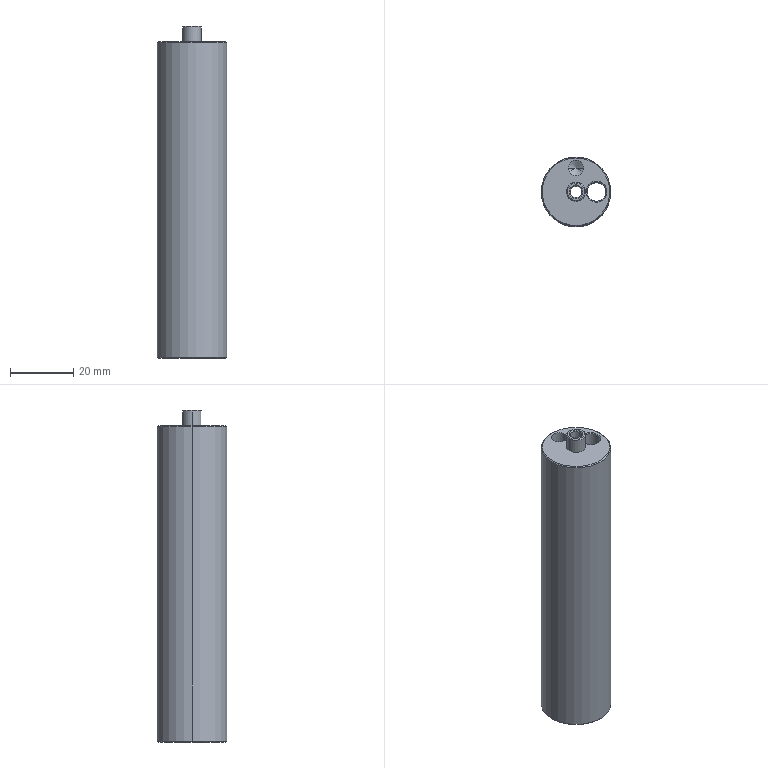Part | SolidWorks | features ICE 3, Chamfer 1, Extrusion 1, HoleWzd 1 | 1 solid | 29 faces | box 22 x 22 x 105 mm | volume 33982 mm3 | cone 16 | cylinder 10 | plane 3 | commonest cylinder face diameters 6 x4 3.7 x2 5 x2 22 x2
STEP:
#1=CARTESIAN_POINT('',(10.7,0.,100.));
#2=VERTEX_POINT('',#1);
#3=CARTESIAN_POINT('',(-10.7,0.,100.));
#4=VERTEX_POINT('',#3);
#5=CARTESIAN_POINT('',(0.,0.,100.));
#6=DIRECTION('',(0.,0.,1.));
#7=DIRECTION('',(1.,0.,0.));
#8=AXIS2_PLACEMENT_3D('',#5,#6,#7);
#9=CIRCLE('',#8,10.7);
#10=EDGE_CURVE('',#2,#4,#9,.T.);
#11=ORIENTED_EDGE('',*,*,#10,.F.);
#12=CARTESIAN_POINT('',(11.,0.,99.7));
#13=VERTEX_POINT('',#12);
#14=CARTESIAN_POINT('',(10.7,0.,100.));
#15=DIRECTION('',(0.7071,0.,-0.7071));
#16=VECTOR('',#15,1000.);
#17=LINE('',#14,#16);
#18=EDGE_CURVE('',#2,#13,#17,.T.);
#19=ORIENTED_EDGE('',*,*,#18,.T.);
#20=CARTESIAN_POINT('',(-11.,0.,99.7));
#21=VERTEX_POINT('',#20);
#22=CARTESIAN_POINT('',(0.,0.,99.7));
#23=DIRECTION('',(0.,0.,-1.));
#24=DIRECTION('',(1.,0.,0.));
#25=AXIS2_PLACEMENT_3D('',#22,#23,#24);
#26=CIRCLE('',#25,11.);
#27=EDGE_CURVE('',#21,#13,#26,.T.);
#28=ORIENTED_EDGE('',*,*,#27,.F.);
#29=CARTESIAN_POINT('',(-10.7,0.,100.));
#30=DIRECTION('',(-0.7071,0.,-0.7071));
#31=VECTOR('',#30,1000.);
#32=LINE('',#29,#31);
#33=EDGE_CURVE('',#4,#21,#32,.T.);
#34=ORIENTED_EDGE('',*,*,#33,.F.);
#35=EDGE_LOOP('',(#11,#19,#28,#34));
#36=FACE_OUTER_BOUND('',#35,.T.);
#37=CARTESIAN_POINT('',(0.,0.,100.));
#38=DIRECTION('',(0.,0.,-1.));
#39=DIRECTION('',(-1.,0.,0.));
#40=AXIS2_PLACEMENT_3D('',#37,#38,#39);
#41=CONICAL_SURFACE('',#40,10.7,0.7854);
#42=ADVANCED_FACE('',(#36),#41,.T.);
#43=CARTESIAN_POINT('',(-10.7,0.,0.));
#44=VERTEX_POINT('',#43);
#45=CARTESIAN_POINT('',(10.7,0.,0.));
#46=VERTEX_POINT('',#45);
#47=CARTESIAN_POINT('',(0.,0.,0.));
#48=DIRECTION('',(0.,0.,-1.));
#49=DIRECTION('',(1.,0.,0.));
#50=AXIS2_PLACEMENT_3D('',#47,#48,#49);
#51=CIRCLE('',#50,10.7);
#52=EDGE_CURVE('',#44,#46,#51,.T.);
#53=ORIENTED_EDGE('',*,*,#52,.F.);
#54=CARTESIAN_POINT('',(-11.,0.,0.3));
#55=VERTEX_POINT('',#54);
#56=CARTESIAN_POINT('',(-11.,0.,0.3));
#57=DIRECTION('',(-0.7071,0.,0.7071));
#58=VECTOR('',#57,1000.);
#59=LINE('',#56,#58);
#60=EDGE_CURVE('',#44,#55,#59,.T.);
#61=ORIENTED_EDGE('',*,*,#60,.T.);
#62=CARTESIAN_POINT('',(11.,0.,0.3));
#63=VERTEX_POINT('',#62);
#64=CARTESIAN_POINT('',(0.,0.,0.3));
#65=DIRECTION('',(0.,0.,1.));
#66=DIRECTION('',(1.,0.,0.));
#67=AXIS2_PLACEMENT_3D('',#64,#65,#66);
#68=CIRCLE('',#67,11.);
#69=EDGE_CURVE('',#63,#55,#68,.T.);
#70=ORIENTED_EDGE('',*,*,#69,.F.);
#71=CARTESIAN_POINT('',(11.,0.,0.3));
#72=DIRECTION('',(0.7071,0.,0.7071));
#73=VECTOR('',#72,1000.);
#74=LINE('',#71,#73);
#75=EDGE_CURVE('',#46,#63,#74,.T.);
#76=ORIENTED_EDGE('',*,*,#75,.F.);
#77=EDGE_LOOP('',(#53,#61,#70,#76));
#78=FACE_OUTER_BOUND('',#77,.T.);
#79=CARTESIAN_POINT('',(0.,0.,0.3));
#80=DIRECTION('',(0.,0.,1.));
#81=DIRECTION('',(1.,0.,0.));
#82=AXIS2_PLACEMENT_3D('',#79,#80,#81);
#83=CONICAL_SURFACE('',#82,11.,0.7854);
#84=ADVANCED_FACE('',(#78),#83,.T.);
#85=CARTESIAN_POINT('',(9.5,0.,0.3));
#86=VERTEX_POINT('',#85);
#87=CARTESIAN_POINT('',(3.5,0.,0.3));
#88=VERTEX_POINT('',#87);
#89=CARTESIAN_POINT('',(6.5,0.,0.3));
#90=DIRECTION('',(0.,0.,-1.));
#91=DIRECTION('',(1.,0.,0.));
#92=AXIS2_PLACEMENT_3D('',#89,#90,#91);
#93=CIRCLE('',#92,3.);
#94=EDGE_CURVE('',#86,#88,#93,.T.);
#95=ORIENTED_EDGE('',*,*,#94,.F.);
#96=CARTESIAN_POINT('',(9.8,0.,0.));
#97=VERTEX_POINT('',#96);
#98=CARTESIAN_POINT('',(9.8,0.,0.));
#99=DIRECTION('',(0.7071,0.,-0.7071));
#100=VECTOR('',#99,1000.);
#101=LINE('',#98,#100);
#102=EDGE_CURVE('',#86,#97,#101,.T.);
#103=ORIENTED_EDGE('',*,*,#102,.T.);
#104=CARTESIAN_POINT('',(3.2,0.,0.));
#105=VERTEX_POINT('',#104);
#106=CARTESIAN_POINT('',(6.5,0.,0.));
#107=DIRECTION('',(0.,0.,1.));
#108=DIRECTION('',(1.,0.,0.));
#109=AXIS2_PLACEMENT_3D('',#106,#107,#108);
#110=CIRCLE('',#109,3.3);
#111=EDGE_CURVE('',#105,#97,#110,.T.);
#112=ORIENTED_EDGE('',*,*,#111,.F.);
#113=CARTESIAN_POINT('',(3.2,0.,0.));
#114=DIRECTION('',(-0.7071,0.,-0.7071));
#115=VECTOR('',#114,1000.);
#116=LINE('',#113,#115);
#117=EDGE_CURVE('',#88,#105,#116,.T.);
#118=ORIENTED_EDGE('',*,*,#117,.F.);
#119=EDGE_LOOP('',(#95,#103,#112,#118));
#120=FACE_OUTER_BOUND('',#119,.T.);
#121=CARTESIAN_POINT('',(6.5,0.,0.));
#122=DIRECTION('',(0.,0.,-1.));
#123=DIRECTION('',(-1.,0.,0.));
#124=AXIS2_PLACEMENT_3D('',#121,#122,#123);
#125=CONICAL_SURFACE('',#124,3.3,0.7854);
#126=ADVANCED_FACE('',(#120),#125,.F.);
#127=CARTESIAN_POINT('',(1.85,0.,0.3));
#128=VERTEX_POINT('',#127);
#129=CARTESIAN_POINT('',(-1.85,0.,0.3));
#130=VERTEX_POINT('',#129);
#131=CARTESIAN_POINT('',(0.,0.,0.3));
#132=DIRECTION('',(0.,0.,-1.));
#133=DIRECTION('',(1.,0.,0.));
#134=AXIS2_PLACEMENT_3D('',#131,#132,#133);
#135=CIRCLE('',#134,1.85);
#136=EDGE_CURVE('',#128,#130,#135,.T.);
#137=ORIENTED_EDGE('',*,*,#136,.F.);
#138=CARTESIAN_POINT('',(2.15,0.,0.));
#139=VERTEX_POINT('',#138);
#140=CARTESIAN_POINT('',(2.15,0.,0.));
#141=DIRECTION('',(0.7071,0.,-0.7071));
#142=VECTOR('',#141,1000.);
#143=LINE('',#140,#142);
#144=EDGE_CURVE('',#128,#139,#143,.T.);
#145=ORIENTED_EDGE('',*,*,#144,.T.);
#146=CARTESIAN_POINT('',(-2.15,0.,0.));
#147=VERTEX_POINT('',#146);
#148=CARTESIAN_POINT('',(0.,0.,0.));
#149=DIRECTION('',(0.,0.,1.));
#150=DIRECTION('',(1.,0.,0.));
#151=AXIS2_PLACEMENT_3D('',#148,#149,#150);
#152=CIRCLE('',#151,2.15);
#153=EDGE_CURVE('',#147,#139,#152,.T.);
#154=ORIENTED_EDGE('',*,*,#153,.F.);
#155=CARTESIAN_POINT('',(-2.15,0.,0.));
#156=DIRECTION('',(-0.7071,0.,-0.7071));
#157=VECTOR('',#156,1000.);
#158=LINE('',#155,#157);
#159=EDGE_CURVE('',#130,#147,#158,.T.);
#160=ORIENTED_EDGE('',*,*,#159,.F.);
#161=EDGE_LOOP('',(#137,#145,#154,#160));
#162=FACE_OUTER_BOUND('',#161,.T.);
#163=CARTESIAN_POINT('',(0.,0.,0.));
#164=DIRECTION('',(0.,0.,-1.));
#165=DIRECTION('',(-1.,0.,0.));
#166=AXIS2_PLACEMENT_3D('',#163,#164,#165);
#167=CONICAL_SURFACE('',#166,2.15,0.7854);
#168=ADVANCED_FACE('',(#162),#167,.F.);
#169=CARTESIAN_POINT('',(2.7,0.,105.));
#170=VERTEX_POINT('',#169);
#171=CARTESIAN_POINT('',(-2.7,0.,105.));
#172=VERTEX_POINT('',#171);
#173=CARTESIAN_POINT('',(0.,0.,105.));
#174=DIRECTION('',(0.,0.,1.));
#175=DIRECTION('',(1.,0.,0.));
#176=AXIS2_PLACEMENT_3D('',#173,#174,#175);
#177=CIRCLE('',#176,2.7);
#178=EDGE_CURVE('',#170,#172,#177,.T.);
#179=ORIENTED_EDGE('',*,*,#178,.F.);
#180=CARTESIAN_POINT('',(3.,0.,104.7));
#181=VERTEX_POINT('',#180);
#182=CARTESIAN_POINT('',(2.7,0.,105.));
#183=DIRECTION('',(0.7071,0.,-0.7071));
#184=VECTOR('',#183,1000.);
#185=LINE('',#182,#184);
#186=EDGE_CURVE('',#170,#181,#185,.T.);
#187=ORIENTED_EDGE('',*,*,#186,.T.);
#188=CARTESIAN_POINT('',(-3.,0.,104.7));
#189=VERTEX_POINT('',#188);
#190=CARTESIAN_POINT('',(0.,0.,104.7));
#191=DIRECTION('',(0.,0.,-1.));
#192=DIRECTION('',(1.,0.,0.));
#193=AXIS2_PLACEMENT_3D('',#190,#191,#192);
#194=CIRCLE('',#193,3.);
#195=EDGE_CURVE('',#189,#181,#194,.T.);
#196=ORIENTED_EDGE('',*,*,#195,.F.);
#197=CARTESIAN_POINT('',(-2.7,0.,105.));
#198=DIRECTION('',(-0.7071,0.,-0.7071));
#199=VECTOR('',#198,1000.);
#200=LINE('',#197,#199);
#201=EDGE_CURVE('',#172,#189,#200,.T.);
#202=ORIENTED_EDGE('',*,*,#201,.F.);
#203=EDGE_LOOP('',(#179,#187,#196,#202));
#204=FACE_OUTER_BOUND('',#203,.T.);
#205=CARTESIAN_POINT('',(0.,0.,105.));
#206=DIRECTION('',(0.,0.,-1.));
#207=DIRECTION('',(-1.,0.,0.));
#208=AXIS2_PLACEMENT_3D('',#205,#206,#207);
#209=CONICAL_SURFACE('',#208,2.7,0.7854);
#210=ADVANCED_FACE('',(#204),#209,.T.);
#211=CARTESIAN_POINT('',(-1.85,0.,104.7));
#212=VERTEX_POINT('',#211);
#213=CARTESIAN_POINT('',(1.85,0.,104.7));
#214=VERTEX_POINT('',#213);
#215=CARTESIAN_POINT('',(0.,0.,104.7));
#216=DIRECTION('',(0.,0.,1.));
#217=DIRECTION('',(1.,0.,0.));
#218=AXIS2_PLACEMENT_3D('',#215,#216,#217);
#219=CIRCLE('',#218,1.85);
#220=EDGE_CURVE('',#212,#214,#219,.T.);
#221=ORIENTED_EDGE('',*,*,#220,.F.);
#222=CARTESIAN_POINT('',(-2.15,0.,105.));
#223=VERTEX_POINT('',#222);
#224=CARTESIAN_POINT('',(-1.85,0.,104.7));
#225=DIRECTION('',(-0.7071,0.,0.7071));
#226=VECTOR('',#225,1000.);
#227=LINE('',#224,#226);
#228=EDGE_CURVE('',#212,#223,#227,.T.);
#229=ORIENTED_EDGE('',*,*,#228,.T.);
#230=CARTESIAN_POINT('',(2.15,0.,105.));
#231=VERTEX_POINT('',#230);
#232=CARTESIAN_POINT('',(0.,0.,105.));
#233=DIRECTION('',(0.,0.,-1.));
#234=DIRECTION('',(1.,0.,0.));
#235=AXIS2_PLACEMENT_3D('',#232,#233,#234);
#236=CIRCLE('',#235,2.15);
#237=EDGE_CURVE('',#231,#223,#236,.T.);
#238=ORIENTED_EDGE('',*,*,#237,.F.);
#239=CARTESIAN_POINT('',(1.85,0.,104.7));
#240=DIRECTION('',(0.7071,0.,0.7071));
#241=VECTOR('',#240,1000.);
#242=LINE('',#239,#241);
#243=EDGE_CURVE('',#214,#231,#242,.T.);
#244=ORIENTED_EDGE('',*,*,#243,.F.);
#245=EDGE_LOOP('',(#221,#229,#238,#244));
#246=FACE_OUTER_BOUND('',#245,.T.);
#247=CARTESIAN_POINT('',(0.,0.,104.7));
#248=DIRECTION('',(0.,0.,1.));
#249=DIRECTION('',(1.,0.,0.));
#250=AXIS2_PLACEMENT_3D('',#247,#248,#249);
#251=CONICAL_SURFACE('',#250,1.85,0.7854);
#252=ADVANCED_FACE('',(#246),#251,.F.);
#253=CARTESIAN_POINT('',(3.5,0.,99.7));
#254=VERTEX_POINT('',#253);
#255=CARTESIAN_POINT('',(9.5,0.,99.7));
#256=VERTEX_POINT('',#255);
#257=CARTESIAN_POINT('',(6.5,0.,99.7));
#258=DIRECTION('',(0.,0.,1.));
#259=DIRECTION('',(1.,0.,0.));
#260=AXIS2_PLACEMENT_3D('',#257,#258,#259);
#261=CIRCLE('',#260,3.);
#262=EDGE_CURVE('',#254,#256,#261,.T.);
#263=ORIENTED_EDGE('',*,*,#262,.F.);
#264=CARTESIAN_POINT('',(3.2,0.,100.));
#265=VERTEX_POINT('',#264);
#266=CARTESIAN_POINT('',(3.5,0.,99.7));
#267=DIRECTION('',(-0.7071,0.,0.7071));
#268=VECTOR('',#267,1000.);
#269=LINE('',#266,#268);
#270=EDGE_CURVE('',#254,#265,#269,.T.);
#271=ORIENTED_EDGE('',*,*,#270,.T.);
#272=CARTESIAN_POINT('',(9.8,0.,100.));
#273=VERTEX_POINT('',#272);
#274=CARTESIAN_POINT('',(6.5,0.,100.));
#275=DIRECTION('',(0.,0.,-1.));
#276=DIRECTION('',(1.,0.,0.));
#277=AXIS2_PLACEMENT_3D('',#274,#275,#276);
#278=CIRCLE('',#277,3.3);
#279=EDGE_CURVE('',#273,#265,#278,.T.);
#280=ORIENTED_EDGE('',*,*,#279,.F.);
#281=CARTESIAN_POINT('',(9.5,0.,99.7));
#282=DIRECTION('',(0.7071,0.,0.7071));
#283=VECTOR('',#282,1000.);
#284=LINE('',#281,#283);
#285=EDGE_CURVE('',#256,#273,#284,.T.);
#286=ORIENTED_EDGE('',*,*,#285,.F.);
#287=EDGE_LOOP('',(#263,#271,#280,#286));
#288=FACE_OUTER_BOUND('',#287,.T.);
#289=CARTESIAN_POINT('',(6.5,0.,99.7));
#290=DIRECTION('',(0.,0.,1.));
#291=DIRECTION('',(1.,0.,0.));
#292=AXIS2_PLACEMENT_3D('',#289,#290,#291);
#293=CONICAL_SURFACE('',#292,3.,0.7854);
#294=ADVANCED_FACE('',(#288),#293,.F.);
#295=CARTESIAN_POINT('',(-2.5,7.5,90.));
#296=VERTEX_POINT('',#295);
#297=CARTESIAN_POINT('',(2.5,7.5,90.));
#298=VERTEX_POINT('',#297);
#299=CARTESIAN_POINT('',(0.,7.5,90.));
#300=DIRECTION('',(0.,0.,1.));
#301=DIRECTION('',(1.,0.,0.));
#302=AXIS2_PLACEMENT_3D('',#299,#300,#301);
#303=CIRCLE('',#302,2.5);
#304=EDGE_CURVE('',#296,#298,#303,.T.);
#305=ORIENTED_EDGE('',*,*,#304,.F.);
#306=CARTESIAN_POINT('',(-2.5,7.5,100.));
#307=VERTEX_POINT('',#306);
#308=CARTESIAN_POINT('',(-2.5,7.5,100.));
#309=DIRECTION('',(0.,0.,1.));
#310=VECTOR('',#309,1000.);
#311=LINE('',#308,#310);
#312=EDGE_CURVE('',#296,#307,#311,.T.);
#313=ORIENTED_EDGE('',*,*,#312,.T.);
#314=CARTESIAN_POINT('',(2.5,7.5,100.));
#315=VERTEX_POINT('',#314);
#316=CARTESIAN_POINT('',(0.,7.5,100.));
#317=DIRECTION('',(0.,0.,1.));
#318=DIRECTION('',(1.,0.,0.));
#319=AXIS2_PLACEMENT_3D('',#316,#317,#318);
#320=CIRCLE('',#319,2.5);
#321=EDGE_CURVE('',#307,#315,#320,.T.);
#322=ORIENTED_EDGE('',*,*,#321,.T.);
#323=CARTESIAN_POINT('',(2.5,7.5,100.));
#324=DIRECTION('',(0.,0.,1.));
#325=VECTOR('',#324,1000.);
#326=LINE('',#323,#325);
#327=EDGE_CURVE('',#298,#315,#326,.T.);
#328=ORIENTED_EDGE('',*,*,#327,.F.);
#329=EDGE_LOOP('',(#305,#313,#322,#328));
#330=FACE_OUTER_BOUND('',#329,.T.);
#331=CARTESIAN_POINT('',(0.,7.5,100.));
#332=DIRECTION('',(0.,0.,1.));
#333=DIRECTION('',(1.,0.,0.));
#334=AXIS2_PLACEMENT_3D('',#331,#332,#333);
#335=CYLINDRICAL_SURFACE('',#334,2.5);
#336=ADVANCED_FACE('',(#330),#335,.F.);
#337=CARTESIAN_POINT('',(0.,7.5,88.498));
#338=VERTEX_POINT('',#337);
#339=CARTESIAN_POINT('',(2.5,7.5,90.));
#340=DIRECTION('',(0.8572,0.,0.515));
#341=VECTOR('',#340,1000.);
#342=LINE('',#339,#341);
#343=EDGE_CURVE('',#338,#298,#342,.T.);
#344=ORIENTED_EDGE('',*,*,#343,.F.);
#345=CARTESIAN_POINT('',(-2.5,7.5,90.));
#346=DIRECTION('',(-0.8572,0.,0.515));
#347=VECTOR('',#346,1000.);
#348=LINE('',#345,#347);
#349=EDGE_CURVE('',#338,#296,#348,.T.);
#350=ORIENTED_EDGE('',*,*,#349,.T.);
#351=ORIENTED_EDGE('',*,*,#304,.T.);
#352=EDGE_LOOP('',(#344,#350,#351));
#353=FACE_OUTER_BOUND('',#352,.T.);
#354=CARTESIAN_POINT('',(0.,7.5,90.));
#355=DIRECTION('',(0.,0.,1.));
#356=DIRECTION('',(1.,0.,0.));
#357=AXIS2_PLACEMENT_3D('',#354,#355,#356);
#358=CONICAL_SURFACE('',#357,2.5,1.03);
#359=ADVANCED_FACE('',(#353),#358,.F.);
#360=ORIENTED_EDGE('',*,*,#94,.T.);
#361=CARTESIAN_POINT('',(3.5,0.,0.));
#362=DIRECTION('',(0.,0.,1.));
#363=VECTOR('',#362,1000.);
#364=LINE('',#361,#363);
#365=EDGE_CURVE('',#88,#254,#364,.T.);
#366=ORIENTED_EDGE('',*,*,#365,.T.);
#367=ORIENTED_EDGE('',*,*,#262,.T.);
#368=CARTESIAN_POINT('',(9.5,0.,0.));
#369=DIRECTION('',(0.,0.,1.));
#370=VECTOR('',#369,1000.);
#371=LINE('',#368,#370);
#372=EDGE_CURVE('',#86,#256,#371,.T.);
#373=ORIENTED_EDGE('',*,*,#372,.F.);
#374=EDGE_LOOP('',(#360,#366,#367,#373));
#375=FACE_OUTER_BOUND('',#374,.T.);
#376=CARTESIAN_POINT('',(6.5,0.,0.));
#377=DIRECTION('',(0.,0.,1.));
#378=DIRECTION('',(1.,0.,0.));
#379=AXIS2_PLACEMENT_3D('',#376,#377,#378);
#380=CYLINDRICAL_SURFACE('',#379,3.);
#381=ADVANCED_FACE('',(#375),#380,.F.);
#382=ORIENTED_EDGE('',*,*,#136,.T.);
#383=CARTESIAN_POINT('',(-1.85,0.,0.));
#384=DIRECTION('',(0.,0.,1.));
#385=VECTOR('',#384,1000.);
#386=LINE('',#383,#385);
#387=EDGE_CURVE('',#130,#212,#386,.T.);
#388=ORIENTED_EDGE('',*,*,#387,.T.);
#389=ORIENTED_EDGE('',*,*,#220,.T.);
#390=CARTESIAN_POINT('',(1.85,0.,0.));
#391=DIRECTION('',(0.,0.,1.));
#392=VECTOR('',#391,1000.);
#393=LINE('',#390,#392);
#394=EDGE_CURVE('',#128,#214,#393,.T.);
#395=ORIENTED_EDGE('',*,*,#394,.F.);
#396=EDGE_LOOP('',(#382,#388,#389,#395));
#397=FACE_OUTER_BOUND('',#396,.T.);
#398=CARTESIAN_POINT('',(0.,0.,0.));
#399=DIRECTION('',(0.,0.,1.));
#400=DIRECTION('',(1.,0.,0.));
#401=AXIS2_PLACEMENT_3D('',#398,#399,#400);
#402=CYLINDRICAL_SURFACE('',#401,1.85);
#403=ADVANCED_FACE('',(#397),#402,.F.);
#404=ORIENTED_EDGE('',*,*,#195,.T.);
#405=CARTESIAN_POINT('',(3.,0.,100.));
#406=VERTEX_POINT('',#405);
#407=CARTESIAN_POINT('',(3.,0.,105.));
#408=DIRECTION('',(0.,0.,-1.));
#409=VECTOR('',#408,1000.);
#410=LINE('',#407,#409);
#411=EDGE_CURVE('',#181,#406,#410,.T.);
#412=ORIENTED_EDGE('',*,*,#411,.T.);
#413=CARTESIAN_POINT('',(-3.,0.,100.));
#414=VERTEX_POINT('',#413);
#415=CARTESIAN_POINT('',(0.,0.,100.));
#416=DIRECTION('',(0.,0.,1.));
#417=DIRECTION('',(1.,0.,0.));
#418=AXIS2_PLACEMENT_3D('',#415,#416,#417);
#419=CIRCLE('',#418,3.);
#420=EDGE_CURVE('',#406,#414,#419,.T.);
#421=ORIENTED_EDGE('',*,*,#420,.T.);
#422=CARTESIAN_POINT('',(-3.,0.,105.));
#423=DIRECTION('',(0.,0.,-1.));
#424=VECTOR('',#423,1000.);
#425=LINE('',#422,#424);
#426=EDGE_CURVE('',#189,#414,#425,.T.);
#427=ORIENTED_EDGE('',*,*,#426,.F.);
#428=EDGE_LOOP('',(#404,#412,#421,#427));
#429=FACE_OUTER_BOUND('',#428,.T.);
#430=CARTESIAN_POINT('',(0.,0.,105.));
#431=DIRECTION('',(0.,0.,-1.));
#432=DIRECTION('',(-1.,0.,0.));
#433=AXIS2_PLACEMENT_3D('',#430,#431,#432);
#434=CYLINDRICAL_SURFACE('',#433,3.);
#435=ADVANCED_FACE('',(#429),#434,.T.);
#436=ORIENTED_EDGE('',*,*,#27,.T.);
#437=CARTESIAN_POINT('',(11.,0.,100.));
#438=DIRECTION('',(0.,0.,-1.));
#439=VECTOR('',#438,1000.);
#440=LINE('',#437,#439);
#441=EDGE_CURVE('',#13,#63,#440,.T.);
#442=ORIENTED_EDGE('',*,*,#441,.T.);
#443=ORIENTED_EDGE('',*,*,#69,.T.);
#444=CARTESIAN_POINT('',(-11.,0.,100.));
#445=DIRECTION('',(0.,0.,-1.));
#446=VECTOR('',#445,1000.);
#447=LINE('',#444,#446);
#448=EDGE_CURVE('',#21,#55,#447,.T.);
#449=ORIENTED_EDGE('',*,*,#448,.F.);
#450=EDGE_LOOP('',(#436,#442,#443,#449));
#451=FACE_OUTER_BOUND('',#450,.T.);
#452=CARTESIAN_POINT('',(0.,0.,100.));
#453=DIRECTION('',(0.,0.,-1.));
#454=DIRECTION('',(-1.,0.,0.));
#455=AXIS2_PLACEMENT_3D('',#452,#453,#454);
#456=CYLINDRICAL_SURFACE('',#455,11.);
#457=ADVANCED_FACE('',(#451),#456,.T.);
#458=ORIENTED_EDGE('',*,*,#279,.T.);
#459=CARTESIAN_POINT('',(6.5,0.,100.));
#460=DIRECTION('',(0.,0.,-1.));
#461=DIRECTION('',(1.,0.,0.));
#462=AXIS2_PLACEMENT_3D('',#459,#460,#461);
#463=CIRCLE('',#462,3.3);
#464=EDGE_CURVE('',#265,#273,#463,.T.);
#465=ORIENTED_EDGE('',*,*,#464,.T.);
#466=EDGE_LOOP('',(#458,#465));
#467=FACE_BOUND('',#466,.T.);
#468=CARTESIAN_POINT('',(0.,0.,100.));
#469=DIRECTION('',(0.,0.,1.));
#470=DIRECTION('',(1.,0.,0.));
#471=AXIS2_PLACEMENT_3D('',#468,#469,#470);
#472=CIRCLE('',#471,10.7);
#473=EDGE_CURVE('',#4,#2,#472,.T.);
#474=ORIENTED_EDGE('',*,*,#473,.T.);
#475=ORIENTED_EDGE('',*,*,#10,.T.);
#476=EDGE_LOOP('',(#474,#475));
#477=FACE_OUTER_BOUND('',#476,.T.);
#478=CARTESIAN_POINT('',(0.,7.5,100.));
#479=DIRECTION('',(0.,0.,1.));
#480=DIRECTION('',(1.,0.,0.));
#481=AXIS2_PLACEMENT_3D('',#478,#479,#480);
#482=CIRCLE('',#481,2.5);
#483=EDGE_CURVE('',#315,#307,#482,.T.);
#484=ORIENTED_EDGE('',*,*,#483,.F.);
#485=ORIENTED_EDGE('',*,*,#321,.F.);
#486=EDGE_LOOP('',(#484,#485));
#487=FACE_BOUND('',#486,.T.);
#488=CARTESIAN_POINT('',(0.,0.,100.));
#489=DIRECTION('',(0.,0.,1.));
#490=DIRECTION('',(1.,0.,0.));
#491=AXIS2_PLACEMENT_3D('',#488,#489,#490);
#492=CIRCLE('',#491,3.);
#493=EDGE_CURVE('',#414,#406,#492,.T.);
#494=ORIENTED_EDGE('',*,*,#493,.F.);
#495=ORIENTED_EDGE('',*,*,#420,.F.);
#496=EDGE_LOOP('',(#494,#495));
#497=FACE_BOUND('',#496,.T.);
#498=CARTESIAN_POINT('',(0.,0.,100.));
#499=DIRECTION('',(0.,0.,1.));
#500=DIRECTION('',(1.,0.,0.));
#501=AXIS2_PLACEMENT_3D('',#498,#499,#500);
#502=PLANE('',#501);
#503=ADVANCED_FACE('',(#467,#477,#487,#497),#502,.T.);
#504=ORIENTED_EDGE('',*,*,#441,.F.);
#505=CARTESIAN_POINT('',(0.,0.,99.7));
#506=DIRECTION('',(0.,0.,-1.));
#507=DIRECTION('',(1.,0.,0.));
#508=AXIS2_PLACEMENT_3D('',#505,#506,#507);
#509=CIRCLE('',#508,11.);
#510=EDGE_CURVE('',#13,#21,#509,.T.);
#511=ORIENTED_EDGE('',*,*,#510,.T.);
#512=ORIENTED_EDGE('',*,*,#448,.T.);
#513=CARTESIAN_POINT('',(0.,0.,0.3));
#514=DIRECTION('',(0.,0.,1.));
#515=DIRECTION('',(1.,0.,0.));
#516=AXIS2_PLACEMENT_3D('',#513,#514,#515);
#517=CIRCLE('',#516,11.);
#518=EDGE_CURVE('',#55,#63,#517,.T.);
#519=ORIENTED_EDGE('',*,*,#518,.T.);
#520=EDGE_LOOP('',(#504,#511,#512,#519));
#521=FACE_OUTER_BOUND('',#520,.T.);
#522=CARTESIAN_POINT('',(0.,0.,100.));
#523=DIRECTION('',(0.,0.,-1.));
#524=DIRECTION('',(-1.,0.,0.));
#525=AXIS2_PLACEMENT_3D('',#522,#523,#524);
#526=CYLINDRICAL_SURFACE('',#525,11.);
#527=ADVANCED_FACE('',(#521),#526,.T.);
#528=ORIENTED_EDGE('',*,*,#153,.T.);
#529=CARTESIAN_POINT('',(0.,0.,0.));
#530=DIRECTION('',(0.,0.,1.));
#531=DIRECTION('',(1.,0.,0.));
#532=AXIS2_PLACEMENT_3D('',#529,#530,#531);
#533=CIRCLE('',#532,2.15);
#534=EDGE_CURVE('',#139,#147,#533,.T.);
#535=ORIENTED_EDGE('',*,*,#534,.T.);
#536=EDGE_LOOP('',(#528,#535));
#537=FACE_BOUND('',#536,.T.);
#538=ORIENTED_EDGE('',*,*,#111,.T.);
#539=CARTESIAN_POINT('',(6.5,0.,0.));
#540=DIRECTION('',(0.,0.,1.));
#541=DIRECTION('',(1.,0.,0.));
#542=AXIS2_PLACEMENT_3D('',#539,#540,#541);
#543=CIRCLE('',#542,3.3);
#544=EDGE_CURVE('',#97,#105,#543,.T.);
#545=ORIENTED_EDGE('',*,*,#544,.T.);
#546=EDGE_LOOP('',(#538,#545));
#547=FACE_BOUND('',#546,.T.);
#548=CARTESIAN_POINT('',(0.,0.,0.));
#549=DIRECTION('',(0.,0.,-1.));
#550=DIRECTION('',(1.,0.,0.));
#551=AXIS2_PLACEMENT_3D('',#548,#549,#550);
#552=CIRCLE('',#551,10.7);
#553=EDGE_CURVE('',#46,#44,#552,.T.);
#554=ORIENTED_EDGE('',*,*,#553,.T.);
#555=ORIENTED_EDGE('',*,*,#52,.T.);
#556=EDGE_LOOP('',(#554,#555));
#557=FACE_OUTER_BOUND('',#556,.T.);
#558=CARTESIAN_POINT('',(0.,0.,0.));
#559=DIRECTION('',(0.,0.,1.));
#560=DIRECTION('',(1.,0.,0.));
#561=AXIS2_PLACEMENT_3D('',#558,#559,#560);
#562=PLANE('',#561);
#563=ADVANCED_FACE('',(#537,#547,#557),#562,.F.);
#564=ORIENTED_EDGE('',*,*,#411,.F.);
#565=CARTESIAN_POINT('',(0.,0.,104.7));
#566=DIRECTION('',(0.,0.,-1.));
#567=DIRECTION('',(1.,0.,0.));
#568=AXIS2_PLACEMENT_3D('',#565,#566,#567);
#569=CIRCLE('',#568,3.);
#570=EDGE_CURVE('',#181,#189,#569,.T.);
#571=ORIENTED_EDGE('',*,*,#570,.T.);
#572=ORIENTED_EDGE('',*,*,#426,.T.);
#573=ORIENTED_EDGE('',*,*,#493,.T.);
#574=EDGE_LOOP('',(#564,#571,#572,#573));
#575=FACE_OUTER_BOUND('',#574,.T.);
#576=CARTESIAN_POINT('',(0.,0.,105.));
#577=DIRECTION('',(0.,0.,-1.));
#578=DIRECTION('',(-1.,0.,0.));
#579=AXIS2_PLACEMENT_3D('',#576,#577,#578);
#580=CYLINDRICAL_SURFACE('',#579,3.);
#581=ADVANCED_FACE('',(#575),#580,.T.);
#582=ORIENTED_EDGE('',*,*,#237,.T.);
#583=CARTESIAN_POINT('',(0.,0.,105.));
#584=DIRECTION('',(0.,0.,-1.));
#585=DIRECTION('',(1.,0.,0.));
#586=AXIS2_PLACEMENT_3D('',#583,#584,#585);
#587=CIRCLE('',#586,2.15);
#588=EDGE_CURVE('',#223,#231,#587,.T.);
#589=ORIENTED_EDGE('',*,*,#588,.T.);
#590=EDGE_LOOP('',(#582,#589));
#591=FACE_BOUND('',#590,.T.);
#592=CARTESIAN_POINT('',(0.,0.,105.));
#593=DIRECTION('',(0.,0.,1.));
#594=DIRECTION('',(1.,0.,0.));
#595=AXIS2_PLACEMENT_3D('',#592,#593,#594);
#596=CIRCLE('',#595,2.7);
#597=EDGE_CURVE('',#172,#170,#596,.T.);
#598=ORIENTED_EDGE('',*,*,#597,.T.);
#599=ORIENTED_EDGE('',*,*,#178,.T.);
#600=EDGE_LOOP('',(#598,#599));
#601=FACE_OUTER_BOUND('',#600,.T.);
#602=CARTESIAN_POINT('',(0.,0.,105.));
#603=DIRECTION('',(0.,0.,1.));
#604=DIRECTION('',(1.,0.,0.));
#605=AXIS2_PLACEMENT_3D('',#602,#603,#604);
#606=PLANE('',#605);
#607=ADVANCED_FACE('',(#591,#601),#606,.T.);
#608=ORIENTED_EDGE('',*,*,#387,.F.);
#609=CARTESIAN_POINT('',(0.,0.,0.3));
#610=DIRECTION('',(0.,0.,-1.));
#611=DIRECTION('',(1.,0.,0.));
#612=AXIS2_PLACEMENT_3D('',#609,#610,#611);
#613=CIRCLE('',#612,1.85);
#614=EDGE_CURVE('',#130,#128,#613,.T.);
#615=ORIENTED_EDGE('',*,*,#614,.T.);
#616=ORIENTED_EDGE('',*,*,#394,.T.);
#617=CARTESIAN_POINT('',(0.,0.,104.7));
#618=DIRECTION('',(0.,0.,1.));
#619=DIRECTION('',(1.,0.,0.));
#620=AXIS2_PLACEMENT_3D('',#617,#618,#619);
#621=CIRCLE('',#620,1.85);
#622=EDGE_CURVE('',#214,#212,#621,.T.);
#623=ORIENTED_EDGE('',*,*,#622,.T.);
#624=EDGE_LOOP('',(#608,#615,#616,#623));
#625=FACE_OUTER_BOUND('',#624,.T.);
#626=CARTESIAN_POINT('',(0.,0.,0.));
#627=DIRECTION('',(0.,0.,1.));
#628=DIRECTION('',(1.,0.,0.));
#629=AXIS2_PLACEMENT_3D('',#626,#627,#628);
#630=CYLINDRICAL_SURFACE('',#629,1.85);
#631=ADVANCED_FACE('',(#625),#630,.F.);
#632=ORIENTED_EDGE('',*,*,#365,.F.);
#633=CARTESIAN_POINT('',(6.5,0.,0.3));
#634=DIRECTION('',(0.,0.,-1.));
#635=DIRECTION('',(1.,0.,0.));
#636=AXIS2_PLACEMENT_3D('',#633,#634,#635);
#637=CIRCLE('',#636,3.);
#638=EDGE_CURVE('',#88,#86,#637,.T.);
#639=ORIENTED_EDGE('',*,*,#638,.T.);
#640=ORIENTED_EDGE('',*,*,#372,.T.);
#641=CARTESIAN_POINT('',(6.5,0.,99.7));
#642=DIRECTION('',(0.,0.,1.));
#643=DIRECTION('',(1.,0.,0.));
#644=AXIS2_PLACEMENT_3D('',#641,#642,#643);
#645=CIRCLE('',#644,3.);
#646=EDGE_CURVE('',#256,#254,#645,.T.);
#647=ORIENTED_EDGE('',*,*,#646,.T.);
#648=EDGE_LOOP('',(#632,#639,#640,#647));
#649=FACE_OUTER_BOUND('',#648,.T.);
#650=CARTESIAN_POINT('',(6.5,0.,0.));
#651=DIRECTION('',(0.,0.,1.));
#652=DIRECTION('',(1.,0.,0.));
#653=AXIS2_PLACEMENT_3D('',#650,#651,#652);
#654=CYLINDRICAL_SURFACE('',#653,3.);
#655=ADVANCED_FACE('',(#649),#654,.F.);
#656=ORIENTED_EDGE('',*,*,#349,.F.);
#657=ORIENTED_EDGE('',*,*,#343,.T.);
#658=CARTESIAN_POINT('',(0.,7.5,90.));
#659=DIRECTION('',(0.,0.,1.));
#660=DIRECTION('',(1.,0.,0.));
#661=AXIS2_PLACEMENT_3D('',#658,#659,#660);
#662=CIRCLE('',#661,2.5);
#663=EDGE_CURVE('',#298,#296,#662,.T.);
#664=ORIENTED_EDGE('',*,*,#663,.T.);
#665=EDGE_LOOP('',(#656,#657,#664));
#666=FACE_OUTER_BOUND('',#665,.T.);
#667=CARTESIAN_POINT('',(0.,7.5,90.));
#668=DIRECTION('',(0.,0.,1.));
#669=DIRECTION('',(1.,0.,0.));
#670=AXIS2_PLACEMENT_3D('',#667,#668,#669);
#671=CONICAL_SURFACE('',#670,2.5,1.03);
#672=ADVANCED_FACE('',(#666),#671,.F.);
#673=ORIENTED_EDGE('',*,*,#312,.F.);
#674=ORIENTED_EDGE('',*,*,#663,.F.);
#675=ORIENTED_EDGE('',*,*,#327,.T.);
#676=ORIENTED_EDGE('',*,*,#483,.T.);
#677=EDGE_LOOP('',(#673,#674,#675,#676));
#678=FACE_OUTER_BOUND('',#677,.T.);
#679=CARTESIAN_POINT('',(0.,7.5,100.));
#680=DIRECTION('',(0.,0.,1.));
#681=DIRECTION('',(1.,0.,0.));
#682=AXIS2_PLACEMENT_3D('',#679,#680,#681);
#683=CYLINDRICAL_SURFACE('',#682,2.5);
#684=ADVANCED_FACE('',(#678),#683,.F.);
#685=ORIENTED_EDGE('',*,*,#270,.F.);
#686=ORIENTED_EDGE('',*,*,#646,.F.);
#687=ORIENTED_EDGE('',*,*,#285,.T.);
#688=ORIENTED_EDGE('',*,*,#464,.F.);
#689=EDGE_LOOP('',(#685,#686,#687,#688));
#690=FACE_OUTER_BOUND('',#689,.T.);
#691=CARTESIAN_POINT('',(6.5,0.,99.7));
#692=DIRECTION('',(0.,0.,1.));
#693=DIRECTION('',(1.,0.,0.));
#694=AXIS2_PLACEMENT_3D('',#691,#692,#693);
#695=CONICAL_SURFACE('',#694,3.,0.7854);
#696=ADVANCED_FACE('',(#690),#695,.F.);
#697=ORIENTED_EDGE('',*,*,#228,.F.);
#698=ORIENTED_EDGE('',*,*,#622,.F.);
#699=ORIENTED_EDGE('',*,*,#243,.T.);
#700=ORIENTED_EDGE('',*,*,#588,.F.);
#701=EDGE_LOOP('',(#697,#698,#699,#700));
#702=FACE_OUTER_BOUND('',#701,.T.);
#703=CARTESIAN_POINT('',(0.,0.,104.7));
#704=DIRECTION('',(0.,0.,1.));
#705=DIRECTION('',(1.,0.,0.));
#706=AXIS2_PLACEMENT_3D('',#703,#704,#705);
#707=CONICAL_SURFACE('',#706,1.85,0.7854);
#708=ADVANCED_FACE('',(#702),#707,.F.);
#709=ORIENTED_EDGE('',*,*,#186,.F.);
#710=ORIENTED_EDGE('',*,*,#597,.F.);
#711=ORIENTED_EDGE('',*,*,#201,.T.);
#712=ORIENTED_EDGE('',*,*,#570,.F.);
#713=EDGE_LOOP('',(#709,#710,#711,#712));
#714=FACE_OUTER_BOUND('',#713,.T.);
#715=CARTESIAN_POINT('',(0.,0.,105.));
#716=DIRECTION('',(0.,0.,-1.));
#717=DIRECTION('',(-1.,0.,0.));
#718=AXIS2_PLACEMENT_3D('',#715,#716,#717);
#719=CONICAL_SURFACE('',#718,2.7,0.7854);
#720=ADVANCED_FACE('',(#714),#719,.T.);
#721=ORIENTED_EDGE('',*,*,#144,.F.);
#722=ORIENTED_EDGE('',*,*,#614,.F.);
#723=ORIENTED_EDGE('',*,*,#159,.T.);
#724=ORIENTED_EDGE('',*,*,#534,.F.);
#725=EDGE_LOOP('',(#721,#722,#723,#724));
#726=FACE_OUTER_BOUND('',#725,.T.);
#727=CARTESIAN_POINT('',(0.,0.,0.));
#728=DIRECTION('',(0.,0.,-1.));
#729=DIRECTION('',(-1.,0.,0.));
#730=AXIS2_PLACEMENT_3D('',#727,#728,#729);
#731=CONICAL_SURFACE('',#730,2.15,0.7854);
#732=ADVANCED_FACE('',(#726),#731,.F.);
#733=ORIENTED_EDGE('',*,*,#102,.F.);
#734=ORIENTED_EDGE('',*,*,#638,.F.);
#735=ORIENTED_EDGE('',*,*,#117,.T.);
#736=ORIENTED_EDGE('',*,*,#544,.F.);
#737=EDGE_LOOP('',(#733,#734,#735,#736));
#738=FACE_OUTER_BOUND('',#737,.T.);
#739=CARTESIAN_POINT('',(6.5,0.,0.));
#740=DIRECTION('',(0.,0.,-1.));
#741=DIRECTION('',(-1.,0.,0.));
#742=AXIS2_PLACEMENT_3D('',#739,#740,#741);
#743=CONICAL_SURFACE('',#742,3.3,0.7854);
#744=ADVANCED_FACE('',(#738),#743,.F.);
#745=ORIENTED_EDGE('',*,*,#60,.F.);
#746=ORIENTED_EDGE('',*,*,#553,.F.);
#747=ORIENTED_EDGE('',*,*,#75,.T.);
#748=ORIENTED_EDGE('',*,*,#518,.F.);
#749=EDGE_LOOP('',(#745,#746,#747,#748));
#750=FACE_OUTER_BOUND('',#749,.T.);
#751=CARTESIAN_POINT('',(0.,0.,0.3));
#752=DIRECTION('',(0.,0.,1.));
#753=DIRECTION('',(1.,0.,0.));
#754=AXIS2_PLACEMENT_3D('',#751,#752,#753);
#755=CONICAL_SURFACE('',#754,11.,0.7854);
#756=ADVANCED_FACE('',(#750),#755,.T.);
#757=ORIENTED_EDGE('',*,*,#18,.F.);
#758=ORIENTED_EDGE('',*,*,#473,.F.);
#759=ORIENTED_EDGE('',*,*,#33,.T.);
#760=ORIENTED_EDGE('',*,*,#510,.F.);
#761=EDGE_LOOP('',(#757,#758,#759,#760));
#762=FACE_OUTER_BOUND('',#761,.T.);
#763=CARTESIAN_POINT('',(0.,0.,100.));
#764=DIRECTION('',(0.,0.,-1.));
#765=DIRECTION('',(-1.,0.,0.));
#766=AXIS2_PLACEMENT_3D('',#763,#764,#765);
#767=CONICAL_SURFACE('',#766,10.7,0.7854);
#768=ADVANCED_FACE('',(#762),#767,.T.);
#769=CLOSED_SHELL('',(#42,#84,#126,#168,#210,#252,#294,#336,#359,#381,#403,#435,#457,#503,#527,#563,#581,#607,#631,#655,#672,#684,#696,#708,#720,#732,#744,#756,#768));
#770=MANIFOLD_SOLID_BREP('',#769);
#771=CARTESIAN_POINT('',(0.,0.,0.));
#772=DIRECTION('',(0.,0.,1.));
#773=DIRECTION('',(1.,0.,0.));
#774=AXIS2_PLACEMENT_3D('',#771,#772,#773);
#775=(LENGTH_UNIT()NAMED_UNIT(*)SI_UNIT(.MILLI.,.METRE.));
#776=UNCERTAINTY_MEASURE_WITH_UNIT(LENGTH_MEASURE(0.00001),#775,'','');
#777=(NAMED_UNIT(*)PLANE_ANGLE_UNIT()SI_UNIT($,.RADIAN.));
#778=(NAMED_UNIT(*)SI_UNIT($,.STERADIAN.)SOLID_ANGLE_UNIT());
#779=(GEOMETRIC_REPRESENTATION_CONTEXT(3)GLOBAL_UNCERTAINTY_ASSIGNED_CONTEXT((#776))GLOBAL_UNIT_ASSIGNED_CONTEXT((#775,#777,#778))REPRESENTATION_CONTEXT('',''));
#780=ADVANCED_BREP_SHAPE_REPRESENTATION('',(#770,#774),#779);